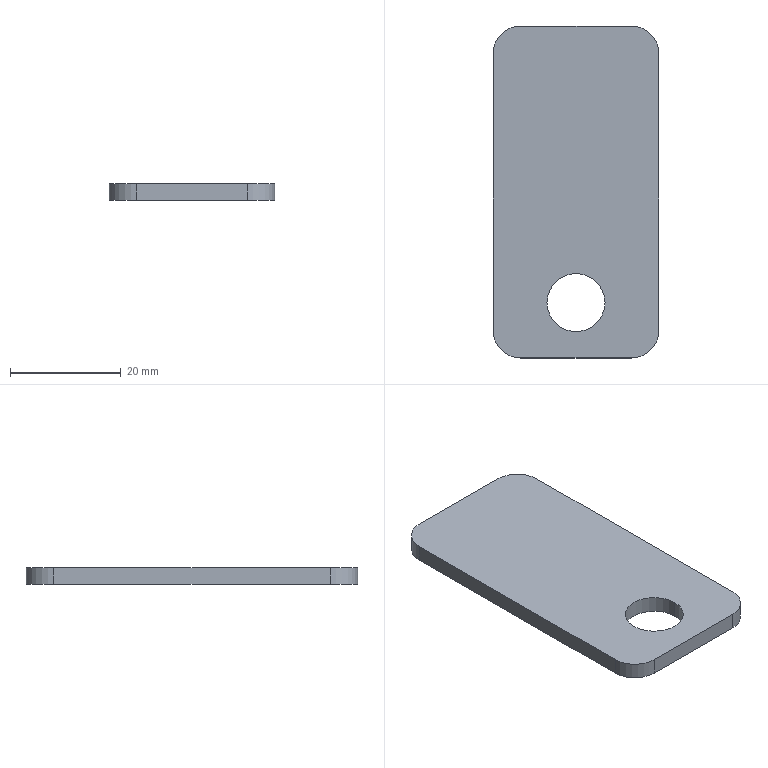Part | SolidWorks | features Extrusion 1 | 1 solid | 12 faces | box 30 x 60 x 3 mm | volume 5076 mm3 | cylinder 6 | plane 6 | commonest cylinder face diameters 10 x4 10.5 x2
STEP:
#1=CARTESIAN_POINT('',(-5.25,-20.,3.));
#2=VERTEX_POINT('',#1);
#3=CARTESIAN_POINT('',(5.25,-20.,3.));
#4=VERTEX_POINT('',#3);
#5=CARTESIAN_POINT('',(0.,-20.,3.));
#6=DIRECTION('',(0.,0.,1.));
#7=DIRECTION('',(1.,0.,0.));
#8=AXIS2_PLACEMENT_3D('',#5,#6,#7);
#9=CIRCLE('',#8,5.25);
#10=EDGE_CURVE('',#2,#4,#9,.T.);
#11=ORIENTED_EDGE('',*,*,#10,.T.);
#12=CARTESIAN_POINT('',(5.25,-20.,0.));
#13=VERTEX_POINT('',#12);
#14=CARTESIAN_POINT('',(5.25,-20.,3.));
#15=DIRECTION('',(0.,0.,-1.));
#16=VECTOR('',#15,1000.);
#17=LINE('',#14,#16);
#18=EDGE_CURVE('',#4,#13,#17,.T.);
#19=ORIENTED_EDGE('',*,*,#18,.T.);
#20=CARTESIAN_POINT('',(-5.25,-20.,0.));
#21=VERTEX_POINT('',#20);
#22=CARTESIAN_POINT('',(0.,-20.,0.));
#23=DIRECTION('',(0.,0.,1.));
#24=DIRECTION('',(1.,0.,0.));
#25=AXIS2_PLACEMENT_3D('',#22,#23,#24);
#26=CIRCLE('',#25,5.25);
#27=EDGE_CURVE('',#21,#13,#26,.T.);
#28=ORIENTED_EDGE('',*,*,#27,.F.);
#29=CARTESIAN_POINT('',(-5.25,-20.,3.));
#30=DIRECTION('',(0.,0.,-1.));
#31=VECTOR('',#30,1000.);
#32=LINE('',#29,#31);
#33=EDGE_CURVE('',#2,#21,#32,.T.);
#34=ORIENTED_EDGE('',*,*,#33,.F.);
#35=EDGE_LOOP('',(#11,#19,#28,#34));
#36=FACE_OUTER_BOUND('',#35,.T.);
#37=CARTESIAN_POINT('',(0.,-20.,3.));
#38=DIRECTION('',(0.,0.,-1.));
#39=DIRECTION('',(-1.,0.,0.));
#40=AXIS2_PLACEMENT_3D('',#37,#38,#39);
#41=CYLINDRICAL_SURFACE('',#40,5.25);
#42=ADVANCED_FACE('',(#36),#41,.F.);
#43=CARTESIAN_POINT('',(15.,25.,3.));
#44=VERTEX_POINT('',#43);
#45=CARTESIAN_POINT('',(10.,30.,3.));
#46=VERTEX_POINT('',#45);
#47=CARTESIAN_POINT('',(10.,25.,3.));
#48=DIRECTION('',(0.,0.,1.));
#49=DIRECTION('',(-1.,0.,0.));
#50=AXIS2_PLACEMENT_3D('',#47,#48,#49);
#51=CIRCLE('',#50,5.);
#52=EDGE_CURVE('',#44,#46,#51,.T.);
#53=ORIENTED_EDGE('',*,*,#52,.T.);
#54=CARTESIAN_POINT('',(-10.,30.,3.));
#55=VERTEX_POINT('',#54);
#56=CARTESIAN_POINT('',(-10.,30.,3.));
#57=DIRECTION('',(-1.,0.,0.));
#58=VECTOR('',#57,1000.);
#59=LINE('',#56,#58);
#60=EDGE_CURVE('',#46,#55,#59,.T.);
#61=ORIENTED_EDGE('',*,*,#60,.T.);
#62=CARTESIAN_POINT('',(-15.,25.,3.));
#63=VERTEX_POINT('',#62);
#64=CARTESIAN_POINT('',(-10.,25.,3.));
#65=DIRECTION('',(0.,0.,1.));
#66=DIRECTION('',(1.,0.,0.));
#67=AXIS2_PLACEMENT_3D('',#64,#65,#66);
#68=CIRCLE('',#67,5.);
#69=EDGE_CURVE('',#55,#63,#68,.T.);
#70=ORIENTED_EDGE('',*,*,#69,.T.);
#71=CARTESIAN_POINT('',(-15.,-25.,3.));
#72=VERTEX_POINT('',#71);
#73=CARTESIAN_POINT('',(-15.,25.,3.));
#74=DIRECTION('',(0.,-1.,0.));
#75=VECTOR('',#74,1000.);
#76=LINE('',#73,#75);
#77=EDGE_CURVE('',#63,#72,#76,.T.);
#78=ORIENTED_EDGE('',*,*,#77,.T.);
#79=CARTESIAN_POINT('',(-10.,-30.,3.));
#80=VERTEX_POINT('',#79);
#81=CARTESIAN_POINT('',(-10.,-25.,3.));
#82=DIRECTION('',(0.,0.,1.));
#83=DIRECTION('',(1.,0.,0.));
#84=AXIS2_PLACEMENT_3D('',#81,#82,#83);
#85=CIRCLE('',#84,5.);
#86=EDGE_CURVE('',#72,#80,#85,.T.);
#87=ORIENTED_EDGE('',*,*,#86,.T.);
#88=CARTESIAN_POINT('',(10.,-30.,3.));
#89=VERTEX_POINT('',#88);
#90=CARTESIAN_POINT('',(-10.,-30.,3.));
#91=DIRECTION('',(1.,0.,0.));
#92=VECTOR('',#91,1000.);
#93=LINE('',#90,#92);
#94=EDGE_CURVE('',#80,#89,#93,.T.);
#95=ORIENTED_EDGE('',*,*,#94,.T.);
#96=CARTESIAN_POINT('',(15.,-25.,3.));
#97=VERTEX_POINT('',#96);
#98=CARTESIAN_POINT('',(10.,-25.,3.));
#99=DIRECTION('',(0.,0.,1.));
#100=DIRECTION('',(1.,0.,0.));
#101=AXIS2_PLACEMENT_3D('',#98,#99,#100);
#102=CIRCLE('',#101,5.);
#103=EDGE_CURVE('',#89,#97,#102,.T.);
#104=ORIENTED_EDGE('',*,*,#103,.T.);
#105=CARTESIAN_POINT('',(15.,25.,3.));
#106=DIRECTION('',(0.,1.,0.));
#107=VECTOR('',#106,1000.);
#108=LINE('',#105,#107);
#109=EDGE_CURVE('',#97,#44,#108,.T.);
#110=ORIENTED_EDGE('',*,*,#109,.T.);
#111=EDGE_LOOP('',(#53,#61,#70,#78,#87,#95,#104,#110));
#112=FACE_OUTER_BOUND('',#111,.T.);
#113=ORIENTED_EDGE('',*,*,#10,.F.);
#114=CARTESIAN_POINT('',(0.,-20.,3.));
#115=DIRECTION('',(0.,0.,1.));
#116=DIRECTION('',(1.,0.,0.));
#117=AXIS2_PLACEMENT_3D('',#114,#115,#116);
#118=CIRCLE('',#117,5.25);
#119=EDGE_CURVE('',#4,#2,#118,.T.);
#120=ORIENTED_EDGE('',*,*,#119,.F.);
#121=EDGE_LOOP('',(#113,#120));
#122=FACE_BOUND('',#121,.T.);
#123=CARTESIAN_POINT('',(10.,25.,3.));
#124=DIRECTION('',(0.,0.,-1.));
#125=DIRECTION('',(-1.,0.,0.));
#126=AXIS2_PLACEMENT_3D('',#123,#124,#125);
#127=PLANE('',#126);
#128=ADVANCED_FACE('',(#112,#122),#127,.F.);
#129=CARTESIAN_POINT('',(15.,25.,0.));
#130=VERTEX_POINT('',#129);
#131=CARTESIAN_POINT('',(10.,30.,0.));
#132=VERTEX_POINT('',#131);
#133=CARTESIAN_POINT('',(10.,25.,0.));
#134=DIRECTION('',(0.,0.,1.));
#135=DIRECTION('',(-1.,0.,0.));
#136=AXIS2_PLACEMENT_3D('',#133,#134,#135);
#137=CIRCLE('',#136,5.);
#138=EDGE_CURVE('',#130,#132,#137,.T.);
#139=ORIENTED_EDGE('',*,*,#138,.F.);
#140=CARTESIAN_POINT('',(15.,-25.,0.));
#141=VERTEX_POINT('',#140);
#142=CARTESIAN_POINT('',(15.,25.,0.));
#143=DIRECTION('',(0.,1.,0.));
#144=VECTOR('',#143,1000.);
#145=LINE('',#142,#144);
#146=EDGE_CURVE('',#141,#130,#145,.T.);
#147=ORIENTED_EDGE('',*,*,#146,.F.);
#148=CARTESIAN_POINT('',(10.,-30.,0.));
#149=VERTEX_POINT('',#148);
#150=CARTESIAN_POINT('',(10.,-25.,0.));
#151=DIRECTION('',(0.,0.,1.));
#152=DIRECTION('',(1.,0.,0.));
#153=AXIS2_PLACEMENT_3D('',#150,#151,#152);
#154=CIRCLE('',#153,5.);
#155=EDGE_CURVE('',#149,#141,#154,.T.);
#156=ORIENTED_EDGE('',*,*,#155,.F.);
#157=CARTESIAN_POINT('',(-10.,-30.,0.));
#158=VERTEX_POINT('',#157);
#159=CARTESIAN_POINT('',(-10.,-30.,0.));
#160=DIRECTION('',(1.,0.,0.));
#161=VECTOR('',#160,1000.);
#162=LINE('',#159,#161);
#163=EDGE_CURVE('',#158,#149,#162,.T.);
#164=ORIENTED_EDGE('',*,*,#163,.F.);
#165=CARTESIAN_POINT('',(-15.,-25.,0.));
#166=VERTEX_POINT('',#165);
#167=CARTESIAN_POINT('',(-10.,-25.,0.));
#168=DIRECTION('',(0.,0.,1.));
#169=DIRECTION('',(1.,0.,0.));
#170=AXIS2_PLACEMENT_3D('',#167,#168,#169);
#171=CIRCLE('',#170,5.);
#172=EDGE_CURVE('',#166,#158,#171,.T.);
#173=ORIENTED_EDGE('',*,*,#172,.F.);
#174=CARTESIAN_POINT('',(-15.,25.,0.));
#175=VERTEX_POINT('',#174);
#176=CARTESIAN_POINT('',(-15.,25.,0.));
#177=DIRECTION('',(0.,-1.,0.));
#178=VECTOR('',#177,1000.);
#179=LINE('',#176,#178);
#180=EDGE_CURVE('',#175,#166,#179,.T.);
#181=ORIENTED_EDGE('',*,*,#180,.F.);
#182=CARTESIAN_POINT('',(-10.,30.,0.));
#183=VERTEX_POINT('',#182);
#184=CARTESIAN_POINT('',(-10.,25.,0.));
#185=DIRECTION('',(0.,0.,1.));
#186=DIRECTION('',(1.,0.,0.));
#187=AXIS2_PLACEMENT_3D('',#184,#185,#186);
#188=CIRCLE('',#187,5.);
#189=EDGE_CURVE('',#183,#175,#188,.T.);
#190=ORIENTED_EDGE('',*,*,#189,.F.);
#191=CARTESIAN_POINT('',(-10.,30.,0.));
#192=DIRECTION('',(-1.,0.,0.));
#193=VECTOR('',#192,1000.);
#194=LINE('',#191,#193);
#195=EDGE_CURVE('',#132,#183,#194,.T.);
#196=ORIENTED_EDGE('',*,*,#195,.F.);
#197=EDGE_LOOP('',(#139,#147,#156,#164,#173,#181,#190,#196));
#198=FACE_OUTER_BOUND('',#197,.T.);
#199=ORIENTED_EDGE('',*,*,#27,.T.);
#200=CARTESIAN_POINT('',(0.,-20.,0.));
#201=DIRECTION('',(0.,0.,1.));
#202=DIRECTION('',(1.,0.,0.));
#203=AXIS2_PLACEMENT_3D('',#200,#201,#202);
#204=CIRCLE('',#203,5.25);
#205=EDGE_CURVE('',#13,#21,#204,.T.);
#206=ORIENTED_EDGE('',*,*,#205,.T.);
#207=EDGE_LOOP('',(#199,#206));
#208=FACE_BOUND('',#207,.T.);
#209=CARTESIAN_POINT('',(10.,25.,0.));
#210=DIRECTION('',(0.,0.,-1.));
#211=DIRECTION('',(-1.,0.,0.));
#212=AXIS2_PLACEMENT_3D('',#209,#210,#211);
#213=PLANE('',#212);
#214=ADVANCED_FACE('',(#198,#208),#213,.T.);
#215=ORIENTED_EDGE('',*,*,#138,.T.);
#216=CARTESIAN_POINT('',(10.,30.,3.));
#217=DIRECTION('',(0.,0.,-1.));
#218=VECTOR('',#217,1000.);
#219=LINE('',#216,#218);
#220=EDGE_CURVE('',#46,#132,#219,.T.);
#221=ORIENTED_EDGE('',*,*,#220,.F.);
#222=ORIENTED_EDGE('',*,*,#52,.F.);
#223=CARTESIAN_POINT('',(15.,25.,3.));
#224=DIRECTION('',(0.,0.,-1.));
#225=VECTOR('',#224,1000.);
#226=LINE('',#223,#225);
#227=EDGE_CURVE('',#44,#130,#226,.T.);
#228=ORIENTED_EDGE('',*,*,#227,.T.);
#229=EDGE_LOOP('',(#215,#221,#222,#228));
#230=FACE_OUTER_BOUND('',#229,.T.);
#231=CARTESIAN_POINT('',(10.,25.,3.));
#232=DIRECTION('',(0.,0.,-1.));
#233=DIRECTION('',(-1.,0.,0.));
#234=AXIS2_PLACEMENT_3D('',#231,#232,#233);
#235=CYLINDRICAL_SURFACE('',#234,5.);
#236=ADVANCED_FACE('',(#230),#235,.T.);
#237=ORIENTED_EDGE('',*,*,#195,.T.);
#238=CARTESIAN_POINT('',(-10.,30.,3.));
#239=DIRECTION('',(0.,0.,-1.));
#240=VECTOR('',#239,1000.);
#241=LINE('',#238,#240);
#242=EDGE_CURVE('',#55,#183,#241,.T.);
#243=ORIENTED_EDGE('',*,*,#242,.F.);
#244=ORIENTED_EDGE('',*,*,#60,.F.);
#245=ORIENTED_EDGE('',*,*,#220,.T.);
#246=EDGE_LOOP('',(#237,#243,#244,#245));
#247=FACE_OUTER_BOUND('',#246,.T.);
#248=CARTESIAN_POINT('',(-10.,30.,3.));
#249=DIRECTION('',(0.,-1.,0.));
#250=DIRECTION('',(1.,0.,0.));
#251=AXIS2_PLACEMENT_3D('',#248,#249,#250);
#252=PLANE('',#251);
#253=ADVANCED_FACE('',(#247),#252,.F.);
#254=ORIENTED_EDGE('',*,*,#189,.T.);
#255=CARTESIAN_POINT('',(-15.,25.,3.));
#256=DIRECTION('',(0.,0.,-1.));
#257=VECTOR('',#256,1000.);
#258=LINE('',#255,#257);
#259=EDGE_CURVE('',#63,#175,#258,.T.);
#260=ORIENTED_EDGE('',*,*,#259,.F.);
#261=ORIENTED_EDGE('',*,*,#69,.F.);
#262=ORIENTED_EDGE('',*,*,#242,.T.);
#263=EDGE_LOOP('',(#254,#260,#261,#262));
#264=FACE_OUTER_BOUND('',#263,.T.);
#265=CARTESIAN_POINT('',(-10.,25.,3.));
#266=DIRECTION('',(0.,0.,-1.));
#267=DIRECTION('',(-1.,0.,0.));
#268=AXIS2_PLACEMENT_3D('',#265,#266,#267);
#269=CYLINDRICAL_SURFACE('',#268,5.);
#270=ADVANCED_FACE('',(#264),#269,.T.);
#271=ORIENTED_EDGE('',*,*,#180,.T.);
#272=CARTESIAN_POINT('',(-15.,-25.,3.));
#273=DIRECTION('',(0.,0.,-1.));
#274=VECTOR('',#273,1000.);
#275=LINE('',#272,#274);
#276=EDGE_CURVE('',#72,#166,#275,.T.);
#277=ORIENTED_EDGE('',*,*,#276,.F.);
#278=ORIENTED_EDGE('',*,*,#77,.F.);
#279=ORIENTED_EDGE('',*,*,#259,.T.);
#280=EDGE_LOOP('',(#271,#277,#278,#279));
#281=FACE_OUTER_BOUND('',#280,.T.);
#282=CARTESIAN_POINT('',(-15.,25.,3.));
#283=DIRECTION('',(1.,0.,0.));
#284=DIRECTION('',(0.,1.,0.));
#285=AXIS2_PLACEMENT_3D('',#282,#283,#284);
#286=PLANE('',#285);
#287=ADVANCED_FACE('',(#281),#286,.F.);
#288=ORIENTED_EDGE('',*,*,#172,.T.);
#289=CARTESIAN_POINT('',(-10.,-30.,3.));
#290=DIRECTION('',(0.,0.,-1.));
#291=VECTOR('',#290,1000.);
#292=LINE('',#289,#291);
#293=EDGE_CURVE('',#80,#158,#292,.T.);
#294=ORIENTED_EDGE('',*,*,#293,.F.);
#295=ORIENTED_EDGE('',*,*,#86,.F.);
#296=ORIENTED_EDGE('',*,*,#276,.T.);
#297=EDGE_LOOP('',(#288,#294,#295,#296));
#298=FACE_OUTER_BOUND('',#297,.T.);
#299=CARTESIAN_POINT('',(-10.,-25.,3.));
#300=DIRECTION('',(0.,0.,-1.));
#301=DIRECTION('',(-1.,0.,0.));
#302=AXIS2_PLACEMENT_3D('',#299,#300,#301);
#303=CYLINDRICAL_SURFACE('',#302,5.);
#304=ADVANCED_FACE('',(#298),#303,.T.);
#305=ORIENTED_EDGE('',*,*,#163,.T.);
#306=CARTESIAN_POINT('',(10.,-30.,3.));
#307=DIRECTION('',(0.,0.,-1.));
#308=VECTOR('',#307,1000.);
#309=LINE('',#306,#308);
#310=EDGE_CURVE('',#89,#149,#309,.T.);
#311=ORIENTED_EDGE('',*,*,#310,.F.);
#312=ORIENTED_EDGE('',*,*,#94,.F.);
#313=ORIENTED_EDGE('',*,*,#293,.T.);
#314=EDGE_LOOP('',(#305,#311,#312,#313));
#315=FACE_OUTER_BOUND('',#314,.T.);
#316=CARTESIAN_POINT('',(-10.,-30.,3.));
#317=DIRECTION('',(0.,1.,0.));
#318=DIRECTION('',(0.,0.,1.));
#319=AXIS2_PLACEMENT_3D('',#316,#317,#318);
#320=PLANE('',#319);
#321=ADVANCED_FACE('',(#315),#320,.F.);
#322=ORIENTED_EDGE('',*,*,#155,.T.);
#323=CARTESIAN_POINT('',(15.,-25.,3.));
#324=DIRECTION('',(0.,0.,-1.));
#325=VECTOR('',#324,1000.);
#326=LINE('',#323,#325);
#327=EDGE_CURVE('',#97,#141,#326,.T.);
#328=ORIENTED_EDGE('',*,*,#327,.F.);
#329=ORIENTED_EDGE('',*,*,#103,.F.);
#330=ORIENTED_EDGE('',*,*,#310,.T.);
#331=EDGE_LOOP('',(#322,#328,#329,#330));
#332=FACE_OUTER_BOUND('',#331,.T.);
#333=CARTESIAN_POINT('',(10.,-25.,3.));
#334=DIRECTION('',(0.,0.,-1.));
#335=DIRECTION('',(-1.,0.,0.));
#336=AXIS2_PLACEMENT_3D('',#333,#334,#335);
#337=CYLINDRICAL_SURFACE('',#336,5.);
#338=ADVANCED_FACE('',(#332),#337,.T.);
#339=ORIENTED_EDGE('',*,*,#146,.T.);
#340=ORIENTED_EDGE('',*,*,#227,.F.);
#341=ORIENTED_EDGE('',*,*,#109,.F.);
#342=ORIENTED_EDGE('',*,*,#327,.T.);
#343=EDGE_LOOP('',(#339,#340,#341,#342));
#344=FACE_OUTER_BOUND('',#343,.T.);
#345=CARTESIAN_POINT('',(15.,25.,3.));
#346=DIRECTION('',(-1.,0.,0.));
#347=DIRECTION('',(0.,-1.,0.));
#348=AXIS2_PLACEMENT_3D('',#345,#346,#347);
#349=PLANE('',#348);
#350=ADVANCED_FACE('',(#344),#349,.F.);
#351=ORIENTED_EDGE('',*,*,#18,.F.);
#352=ORIENTED_EDGE('',*,*,#119,.T.);
#353=ORIENTED_EDGE('',*,*,#33,.T.);
#354=ORIENTED_EDGE('',*,*,#205,.F.);
#355=EDGE_LOOP('',(#351,#352,#353,#354));
#356=FACE_OUTER_BOUND('',#355,.T.);
#357=CARTESIAN_POINT('',(0.,-20.,3.));
#358=DIRECTION('',(0.,0.,-1.));
#359=DIRECTION('',(-1.,0.,0.));
#360=AXIS2_PLACEMENT_3D('',#357,#358,#359);
#361=CYLINDRICAL_SURFACE('',#360,5.25);
#362=ADVANCED_FACE('',(#356),#361,.F.);
#363=CLOSED_SHELL('',(#42,#128,#214,#236,#253,#270,#287,#304,#321,#338,#350,#362));
#364=MANIFOLD_SOLID_BREP('',#363);
#365=CARTESIAN_POINT('',(0.,0.,0.));
#366=DIRECTION('',(0.,0.,1.));
#367=DIRECTION('',(1.,0.,0.));
#368=AXIS2_PLACEMENT_3D('',#365,#366,#367);
#369=(LENGTH_UNIT()NAMED_UNIT(*)SI_UNIT(.MILLI.,.METRE.));
#370=UNCERTAINTY_MEASURE_WITH_UNIT(LENGTH_MEASURE(0.00001),#369,'','');
#371=(NAMED_UNIT(*)PLANE_ANGLE_UNIT()SI_UNIT($,.RADIAN.));
#372=(NAMED_UNIT(*)SI_UNIT($,.STERADIAN.)SOLID_ANGLE_UNIT());
#373=(GEOMETRIC_REPRESENTATION_CONTEXT(3)GLOBAL_UNCERTAINTY_ASSIGNED_CONTEXT((#370))GLOBAL_UNIT_ASSIGNED_CONTEXT((#369,#371,#372))REPRESENTATION_CONTEXT('',''));
#374=ADVANCED_BREP_SHAPE_REPRESENTATION('',(#364,#368),#373);